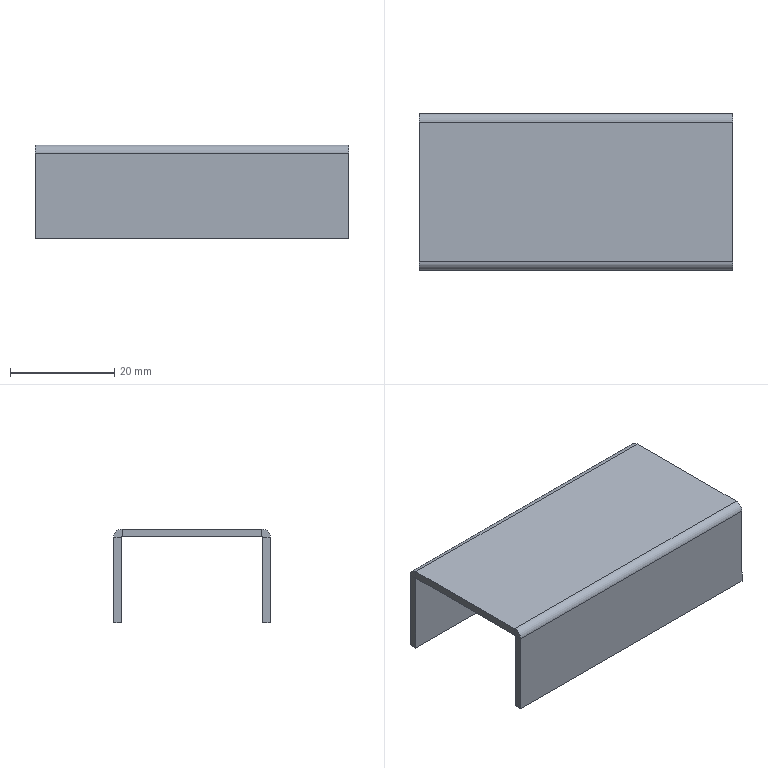Part | SolidWorks | features EdgeFlange 1, FlatPattern 1, SMBaseFlange 1, SheetMetal 1 | 1 solid | 22 faces | box 60 x 30 x 18 mm | volume 5604 mm3 | plane 18 | cylinder 4 | commonest cylinder face diameters 0.2 x2 3.2 x2
STEP:
#1=CARTESIAN_POINT('',(30.,13.4,-1.5));
#2=VERTEX_POINT('',#1);
#3=CARTESIAN_POINT('',(-30.,13.4,-1.5));
#4=VERTEX_POINT('',#3);
#5=CARTESIAN_POINT('',(30.,13.4,-1.5));
#6=DIRECTION('',(-1.,0.,0.));
#7=VECTOR('',#6,1000.);
#8=LINE('',#5,#7);
#9=EDGE_CURVE('',#2,#4,#8,.T.);
#10=ORIENTED_EDGE('',*,*,#9,.F.);
#11=CARTESIAN_POINT('',(30.,-13.4,-1.5));
#12=VERTEX_POINT('',#11);
#13=CARTESIAN_POINT('',(30.,15.,-1.5));
#14=DIRECTION('',(0.,1.,0.));
#15=VECTOR('',#14,1000.);
#16=LINE('',#13,#15);
#17=EDGE_CURVE('',#12,#2,#16,.T.);
#18=ORIENTED_EDGE('',*,*,#17,.F.);
#19=CARTESIAN_POINT('',(-30.,-13.4,-1.5));
#20=VERTEX_POINT('',#19);
#21=CARTESIAN_POINT('',(-30.,-13.4,-1.5));
#22=DIRECTION('',(1.,0.,0.));
#23=VECTOR('',#22,1000.);
#24=LINE('',#21,#23);
#25=EDGE_CURVE('',#20,#12,#24,.T.);
#26=ORIENTED_EDGE('',*,*,#25,.F.);
#27=CARTESIAN_POINT('',(-30.,15.,-1.5));
#28=DIRECTION('',(0.,-1.,0.));
#29=VECTOR('',#28,1000.);
#30=LINE('',#27,#29);
#31=EDGE_CURVE('',#4,#20,#30,.T.);
#32=ORIENTED_EDGE('',*,*,#31,.F.);
#33=EDGE_LOOP('',(#10,#18,#26,#32));
#34=FACE_OUTER_BOUND('',#33,.T.);
#35=CARTESIAN_POINT('',(0.,0.,-1.5));
#36=DIRECTION('',(0.,0.,1.));
#37=DIRECTION('',(1.,0.,0.));
#38=AXIS2_PLACEMENT_3D('',#35,#36,#37);
#39=PLANE('',#38);
#40=ADVANCED_FACE('',(#34),#39,.F.);
#41=CARTESIAN_POINT('',(30.,-13.4,0.));
#42=VERTEX_POINT('',#41);
#43=CARTESIAN_POINT('',(30.,13.4,0.));
#44=VERTEX_POINT('',#43);
#45=CARTESIAN_POINT('',(30.,15.,0.));
#46=DIRECTION('',(0.,1.,0.));
#47=VECTOR('',#46,1000.);
#48=LINE('',#45,#47);
#49=EDGE_CURVE('',#42,#44,#48,.T.);
#50=ORIENTED_EDGE('',*,*,#49,.T.);
#51=CARTESIAN_POINT('',(-30.,13.4,0.));
#52=VERTEX_POINT('',#51);
#53=CARTESIAN_POINT('',(30.,13.4,0.));
#54=DIRECTION('',(-1.,0.,0.));
#55=VECTOR('',#54,1000.);
#56=LINE('',#53,#55);
#57=EDGE_CURVE('',#44,#52,#56,.T.);
#58=ORIENTED_EDGE('',*,*,#57,.T.);
#59=CARTESIAN_POINT('',(-30.,-13.4,0.));
#60=VERTEX_POINT('',#59);
#61=CARTESIAN_POINT('',(-30.,15.,0.));
#62=DIRECTION('',(0.,-1.,0.));
#63=VECTOR('',#62,1000.);
#64=LINE('',#61,#63);
#65=EDGE_CURVE('',#52,#60,#64,.T.);
#66=ORIENTED_EDGE('',*,*,#65,.T.);
#67=CARTESIAN_POINT('',(-30.,-13.4,0.));
#68=DIRECTION('',(1.,0.,0.));
#69=VECTOR('',#68,1000.);
#70=LINE('',#67,#69);
#71=EDGE_CURVE('',#60,#42,#70,.T.);
#72=ORIENTED_EDGE('',*,*,#71,.T.);
#73=EDGE_LOOP('',(#50,#58,#66,#72));
#74=FACE_OUTER_BOUND('',#73,.T.);
#75=CARTESIAN_POINT('',(0.,0.,0.));
#76=DIRECTION('',(0.,0.,1.));
#77=DIRECTION('',(1.,0.,0.));
#78=AXIS2_PLACEMENT_3D('',#75,#76,#77);
#79=PLANE('',#78);
#80=ADVANCED_FACE('',(#74),#79,.T.);
#81=ORIENTED_EDGE('',*,*,#17,.T.);
#82=CARTESIAN_POINT('',(30.,13.4,-1.5));
#83=DIRECTION('',(0.,0.,1.));
#84=VECTOR('',#83,1000.);
#85=LINE('',#82,#84);
#86=EDGE_CURVE('',#2,#44,#85,.T.);
#87=ORIENTED_EDGE('',*,*,#86,.T.);
#88=ORIENTED_EDGE('',*,*,#49,.F.);
#89=CARTESIAN_POINT('',(30.,-13.4,-1.5));
#90=DIRECTION('',(0.,0.,1.));
#91=VECTOR('',#90,1000.);
#92=LINE('',#89,#91);
#93=EDGE_CURVE('',#12,#42,#92,.T.);
#94=ORIENTED_EDGE('',*,*,#93,.F.);
#95=EDGE_LOOP('',(#81,#87,#88,#94));
#96=FACE_OUTER_BOUND('',#95,.T.);
#97=CARTESIAN_POINT('',(30.,15.,-1.5));
#98=DIRECTION('',(1.,0.,0.));
#99=DIRECTION('',(0.,0.,-1.));
#100=AXIS2_PLACEMENT_3D('',#97,#98,#99);
#101=PLANE('',#100);
#102=ADVANCED_FACE('',(#96),#101,.T.);
#103=CARTESIAN_POINT('',(-30.,13.4,-1.5));
#104=DIRECTION('',(0.,0.,1.));
#105=VECTOR('',#104,1000.);
#106=LINE('',#103,#105);
#107=EDGE_CURVE('',#4,#52,#106,.T.);
#108=ORIENTED_EDGE('',*,*,#107,.F.);
#109=ORIENTED_EDGE('',*,*,#31,.T.);
#110=CARTESIAN_POINT('',(-30.,-13.4,-1.5));
#111=DIRECTION('',(0.,0.,1.));
#112=VECTOR('',#111,1000.);
#113=LINE('',#110,#112);
#114=EDGE_CURVE('',#20,#60,#113,.T.);
#115=ORIENTED_EDGE('',*,*,#114,.T.);
#116=ORIENTED_EDGE('',*,*,#65,.F.);
#117=EDGE_LOOP('',(#108,#109,#115,#116));
#118=FACE_OUTER_BOUND('',#117,.T.);
#119=CARTESIAN_POINT('',(-30.,15.,-1.5));
#120=DIRECTION('',(-1.,0.,0.));
#121=DIRECTION('',(0.,0.,1.));
#122=AXIS2_PLACEMENT_3D('',#119,#120,#121);
#123=PLANE('',#122);
#124=ADVANCED_FACE('',(#118),#123,.T.);
#125=CARTESIAN_POINT('',(30.,-13.5,-1.6));
#126=VERTEX_POINT('',#125);
#127=CARTESIAN_POINT('',(30.,-15.,-1.6));
#128=VERTEX_POINT('',#127);
#129=CARTESIAN_POINT('',(30.,-15.,-1.6));
#130=DIRECTION('',(0.,-1.,0.));
#131=VECTOR('',#130,1000.);
#132=LINE('',#129,#131);
#133=EDGE_CURVE('',#126,#128,#132,.T.);
#134=ORIENTED_EDGE('',*,*,#133,.F.);
#135=CARTESIAN_POINT('',(30.,-13.4,-1.6));
#136=DIRECTION('',(1.,0.,0.));
#137=DIRECTION('',(0.,0.,1.));
#138=AXIS2_PLACEMENT_3D('',#135,#136,#137);
#139=CIRCLE('',#138,0.1);
#140=EDGE_CURVE('',#12,#126,#139,.T.);
#141=ORIENTED_EDGE('',*,*,#140,.F.);
#142=ORIENTED_EDGE('',*,*,#93,.T.);
#143=CARTESIAN_POINT('',(30.,-13.4,-1.6));
#144=DIRECTION('',(1.,0.,0.));
#145=DIRECTION('',(0.,0.,1.));
#146=AXIS2_PLACEMENT_3D('',#143,#144,#145);
#147=CIRCLE('',#146,1.6);
#148=EDGE_CURVE('',#42,#128,#147,.T.);
#149=ORIENTED_EDGE('',*,*,#148,.T.);
#150=EDGE_LOOP('',(#134,#141,#142,#149));
#151=FACE_OUTER_BOUND('',#150,.T.);
#152=CARTESIAN_POINT('',(30.,-13.4,-1.6));
#153=DIRECTION('',(1.,0.,0.));
#154=DIRECTION('',(0.,0.,-1.));
#155=AXIS2_PLACEMENT_3D('',#152,#153,#154);
#156=PLANE('',#155);
#157=ADVANCED_FACE('',(#151),#156,.T.);
#158=CARTESIAN_POINT('',(-30.,-13.5,-1.6));
#159=VERTEX_POINT('',#158);
#160=CARTESIAN_POINT('',(-30.,-13.4,-1.6));
#161=DIRECTION('',(-1.,0.,0.));
#162=DIRECTION('',(0.,0.,1.));
#163=AXIS2_PLACEMENT_3D('',#160,#161,#162);
#164=CIRCLE('',#163,0.1);
#165=EDGE_CURVE('',#159,#20,#164,.T.);
#166=ORIENTED_EDGE('',*,*,#165,.F.);
#167=CARTESIAN_POINT('',(-30.,-15.,-1.6));
#168=VERTEX_POINT('',#167);
#169=CARTESIAN_POINT('',(-30.,-13.5,-1.6));
#170=DIRECTION('',(0.,-1.,0.));
#171=VECTOR('',#170,1000.);
#172=LINE('',#169,#171);
#173=EDGE_CURVE('',#159,#168,#172,.T.);
#174=ORIENTED_EDGE('',*,*,#173,.T.);
#175=CARTESIAN_POINT('',(-30.,-13.4,-1.6));
#176=DIRECTION('',(-1.,0.,0.));
#177=DIRECTION('',(0.,0.,1.));
#178=AXIS2_PLACEMENT_3D('',#175,#176,#177);
#179=CIRCLE('',#178,1.6);
#180=EDGE_CURVE('',#168,#60,#179,.T.);
#181=ORIENTED_EDGE('',*,*,#180,.T.);
#182=ORIENTED_EDGE('',*,*,#114,.F.);
#183=EDGE_LOOP('',(#166,#174,#181,#182));
#184=FACE_OUTER_BOUND('',#183,.T.);
#185=CARTESIAN_POINT('',(-30.,-13.4,-1.6));
#186=DIRECTION('',(1.,0.,0.));
#187=DIRECTION('',(0.,0.,-1.));
#188=AXIS2_PLACEMENT_3D('',#185,#186,#187);
#189=PLANE('',#188);
#190=ADVANCED_FACE('',(#184),#189,.F.);
#191=ORIENTED_EDGE('',*,*,#71,.F.);
#192=ORIENTED_EDGE('',*,*,#180,.F.);
#193=CARTESIAN_POINT('',(0.,-15.,-1.6));
#194=DIRECTION('',(-1.,0.,0.));
#195=VECTOR('',#194,1000.);
#196=LINE('',#193,#195);
#197=EDGE_CURVE('',#128,#168,#196,.T.);
#198=ORIENTED_EDGE('',*,*,#197,.F.);
#199=ORIENTED_EDGE('',*,*,#148,.F.);
#200=EDGE_LOOP('',(#191,#192,#198,#199));
#201=FACE_OUTER_BOUND('',#200,.T.);
#202=CARTESIAN_POINT('',(-30.,-13.4,-1.6));
#203=DIRECTION('',(-1.,0.,0.));
#204=DIRECTION('',(0.,-1.,0.));
#205=AXIS2_PLACEMENT_3D('',#202,#203,#204);
#206=CYLINDRICAL_SURFACE('',#205,1.6);
#207=ADVANCED_FACE('',(#201),#206,.T.);
#208=ORIENTED_EDGE('',*,*,#25,.T.);
#209=ORIENTED_EDGE('',*,*,#140,.T.);
#210=CARTESIAN_POINT('',(30.,-13.5,-1.6));
#211=DIRECTION('',(-1.,0.,0.));
#212=VECTOR('',#211,1000.);
#213=LINE('',#210,#212);
#214=EDGE_CURVE('',#126,#159,#213,.T.);
#215=ORIENTED_EDGE('',*,*,#214,.T.);
#216=ORIENTED_EDGE('',*,*,#165,.T.);
#217=EDGE_LOOP('',(#208,#209,#215,#216));
#218=FACE_OUTER_BOUND('',#217,.T.);
#219=CARTESIAN_POINT('',(-30.,-13.4,-1.6));
#220=DIRECTION('',(-1.,0.,0.));
#221=DIRECTION('',(0.,-1.,0.));
#222=AXIS2_PLACEMENT_3D('',#219,#220,#221);
#223=CYLINDRICAL_SURFACE('',#222,0.1);
#224=ADVANCED_FACE('',(#218),#223,.F.);
#225=CARTESIAN_POINT('',(-30.,-15.,-18.));
#226=VERTEX_POINT('',#225);
#227=CARTESIAN_POINT('',(-30.,-15.,-1.5));
#228=DIRECTION('',(0.,0.,1.));
#229=VECTOR('',#228,1000.);
#230=LINE('',#227,#229);
#231=EDGE_CURVE('',#226,#168,#230,.T.);
#232=ORIENTED_EDGE('',*,*,#231,.T.);
#233=ORIENTED_EDGE('',*,*,#173,.F.);
#234=CARTESIAN_POINT('',(-30.,-13.5,-18.));
#235=VERTEX_POINT('',#234);
#236=CARTESIAN_POINT('',(-30.,-13.5,0.));
#237=DIRECTION('',(0.,0.,1.));
#238=VECTOR('',#237,1000.);
#239=LINE('',#236,#238);
#240=EDGE_CURVE('',#235,#159,#239,.T.);
#241=ORIENTED_EDGE('',*,*,#240,.F.);
#242=CARTESIAN_POINT('',(-30.,-15.,-18.));
#243=DIRECTION('',(0.,1.,0.));
#244=VECTOR('',#243,1000.);
#245=LINE('',#242,#244);
#246=EDGE_CURVE('',#226,#235,#245,.T.);
#247=ORIENTED_EDGE('',*,*,#246,.F.);
#248=EDGE_LOOP('',(#232,#233,#241,#247));
#249=FACE_OUTER_BOUND('',#248,.T.);
#250=CARTESIAN_POINT('',(-30.,-15.,-1.5));
#251=DIRECTION('',(-1.,0.,0.));
#252=DIRECTION('',(0.,0.,1.));
#253=AXIS2_PLACEMENT_3D('',#250,#251,#252);
#254=PLANE('',#253);
#255=ADVANCED_FACE('',(#249),#254,.T.);
#256=CARTESIAN_POINT('',(30.,-13.5,-18.));
#257=VERTEX_POINT('',#256);
#258=CARTESIAN_POINT('',(30.,-13.5,0.));
#259=DIRECTION('',(0.,0.,-1.));
#260=VECTOR('',#259,1000.);
#261=LINE('',#258,#260);
#262=EDGE_CURVE('',#126,#257,#261,.T.);
#263=ORIENTED_EDGE('',*,*,#262,.F.);
#264=ORIENTED_EDGE('',*,*,#133,.T.);
#265=CARTESIAN_POINT('',(30.,-15.,-18.));
#266=VERTEX_POINT('',#265);
#267=CARTESIAN_POINT('',(30.,-15.,-18.));
#268=DIRECTION('',(0.,0.,-1.));
#269=VECTOR('',#268,1000.);
#270=LINE('',#267,#269);
#271=EDGE_CURVE('',#128,#266,#270,.T.);
#272=ORIENTED_EDGE('',*,*,#271,.T.);
#273=CARTESIAN_POINT('',(30.,-15.,-18.));
#274=DIRECTION('',(0.,1.,0.));
#275=VECTOR('',#274,1000.);
#276=LINE('',#273,#275);
#277=EDGE_CURVE('',#266,#257,#276,.T.);
#278=ORIENTED_EDGE('',*,*,#277,.T.);
#279=EDGE_LOOP('',(#263,#264,#272,#278));
#280=FACE_OUTER_BOUND('',#279,.T.);
#281=CARTESIAN_POINT('',(30.,-15.,-18.));
#282=DIRECTION('',(1.,0.,0.));
#283=DIRECTION('',(0.,0.,-1.));
#284=AXIS2_PLACEMENT_3D('',#281,#282,#283);
#285=PLANE('',#284);
#286=ADVANCED_FACE('',(#280),#285,.T.);
#287=ORIENTED_EDGE('',*,*,#271,.F.);
#288=ORIENTED_EDGE('',*,*,#197,.T.);
#289=ORIENTED_EDGE('',*,*,#231,.F.);
#290=CARTESIAN_POINT('',(-30.,-15.,-18.));
#291=DIRECTION('',(-1.,0.,0.));
#292=VECTOR('',#291,1000.);
#293=LINE('',#290,#292);
#294=EDGE_CURVE('',#266,#226,#293,.T.);
#295=ORIENTED_EDGE('',*,*,#294,.F.);
#296=EDGE_LOOP('',(#287,#288,#289,#295));
#297=FACE_OUTER_BOUND('',#296,.T.);
#298=CARTESIAN_POINT('',(0.,-15.,0.));
#299=DIRECTION('',(0.,-1.,0.));
#300=DIRECTION('',(0.,0.,-1.));
#301=AXIS2_PLACEMENT_3D('',#298,#299,#300);
#302=PLANE('',#301);
#303=ADVANCED_FACE('',(#297),#302,.T.);
#304=ORIENTED_EDGE('',*,*,#214,.F.);
#305=ORIENTED_EDGE('',*,*,#262,.T.);
#306=CARTESIAN_POINT('',(0.,-13.5,-18.));
#307=DIRECTION('',(-1.,0.,0.));
#308=VECTOR('',#307,1000.);
#309=LINE('',#306,#308);
#310=EDGE_CURVE('',#257,#235,#309,.T.);
#311=ORIENTED_EDGE('',*,*,#310,.T.);
#312=ORIENTED_EDGE('',*,*,#240,.T.);
#313=EDGE_LOOP('',(#304,#305,#311,#312));
#314=FACE_OUTER_BOUND('',#313,.T.);
#315=CARTESIAN_POINT('',(0.,-13.5,0.));
#316=DIRECTION('',(0.,-1.,0.));
#317=DIRECTION('',(0.,0.,-1.));
#318=AXIS2_PLACEMENT_3D('',#315,#316,#317);
#319=PLANE('',#318);
#320=ADVANCED_FACE('',(#314),#319,.F.);
#321=ORIENTED_EDGE('',*,*,#310,.F.);
#322=ORIENTED_EDGE('',*,*,#277,.F.);
#323=ORIENTED_EDGE('',*,*,#294,.T.);
#324=ORIENTED_EDGE('',*,*,#246,.T.);
#325=EDGE_LOOP('',(#321,#322,#323,#324));
#326=FACE_OUTER_BOUND('',#325,.T.);
#327=CARTESIAN_POINT('',(-30.,-15.,-18.));
#328=DIRECTION('',(0.,0.,-1.));
#329=DIRECTION('',(0.,1.,0.));
#330=AXIS2_PLACEMENT_3D('',#327,#328,#329);
#331=PLANE('',#330);
#332=ADVANCED_FACE('',(#326),#331,.T.);
#333=CARTESIAN_POINT('',(-30.,13.5,-1.6));
#334=VERTEX_POINT('',#333);
#335=CARTESIAN_POINT('',(-30.,15.,-1.6));
#336=VERTEX_POINT('',#335);
#337=CARTESIAN_POINT('',(-30.,15.,-1.6));
#338=DIRECTION('',(0.,1.,0.));
#339=VECTOR('',#338,1000.);
#340=LINE('',#337,#339);
#341=EDGE_CURVE('',#334,#336,#340,.T.);
#342=ORIENTED_EDGE('',*,*,#341,.F.);
#343=CARTESIAN_POINT('',(-30.,13.4,-1.6));
#344=DIRECTION('',(-1.,0.,0.));
#345=DIRECTION('',(0.,0.,-1.));
#346=AXIS2_PLACEMENT_3D('',#343,#344,#345);
#347=CIRCLE('',#346,0.1);
#348=EDGE_CURVE('',#4,#334,#347,.T.);
#349=ORIENTED_EDGE('',*,*,#348,.F.);
#350=ORIENTED_EDGE('',*,*,#107,.T.);
#351=CARTESIAN_POINT('',(-30.,13.4,-1.6));
#352=DIRECTION('',(-1.,0.,0.));
#353=DIRECTION('',(0.,0.,-1.));
#354=AXIS2_PLACEMENT_3D('',#351,#352,#353);
#355=CIRCLE('',#354,1.6);
#356=EDGE_CURVE('',#52,#336,#355,.T.);
#357=ORIENTED_EDGE('',*,*,#356,.T.);
#358=EDGE_LOOP('',(#342,#349,#350,#357));
#359=FACE_OUTER_BOUND('',#358,.T.);
#360=CARTESIAN_POINT('',(-30.,13.4,-1.6));
#361=DIRECTION('',(-1.,0.,0.));
#362=DIRECTION('',(0.,0.,1.));
#363=AXIS2_PLACEMENT_3D('',#360,#361,#362);
#364=PLANE('',#363);
#365=ADVANCED_FACE('',(#359),#364,.T.);
#366=CARTESIAN_POINT('',(30.,13.5,-1.6));
#367=VERTEX_POINT('',#366);
#368=CARTESIAN_POINT('',(30.,13.4,-1.6));
#369=DIRECTION('',(1.,0.,0.));
#370=DIRECTION('',(0.,0.,-1.));
#371=AXIS2_PLACEMENT_3D('',#368,#369,#370);
#372=CIRCLE('',#371,0.1);
#373=EDGE_CURVE('',#367,#2,#372,.T.);
#374=ORIENTED_EDGE('',*,*,#373,.F.);
#375=CARTESIAN_POINT('',(30.,15.,-1.6));
#376=VERTEX_POINT('',#375);
#377=CARTESIAN_POINT('',(30.,13.5,-1.6));
#378=DIRECTION('',(0.,1.,0.));
#379=VECTOR('',#378,1000.);
#380=LINE('',#377,#379);
#381=EDGE_CURVE('',#367,#376,#380,.T.);
#382=ORIENTED_EDGE('',*,*,#381,.T.);
#383=CARTESIAN_POINT('',(30.,13.4,-1.6));
#384=DIRECTION('',(1.,0.,0.));
#385=DIRECTION('',(0.,0.,-1.));
#386=AXIS2_PLACEMENT_3D('',#383,#384,#385);
#387=CIRCLE('',#386,1.6);
#388=EDGE_CURVE('',#376,#44,#387,.T.);
#389=ORIENTED_EDGE('',*,*,#388,.T.);
#390=ORIENTED_EDGE('',*,*,#86,.F.);
#391=EDGE_LOOP('',(#374,#382,#389,#390));
#392=FACE_OUTER_BOUND('',#391,.T.);
#393=CARTESIAN_POINT('',(30.,13.4,-1.6));
#394=DIRECTION('',(-1.,0.,0.));
#395=DIRECTION('',(0.,0.,1.));
#396=AXIS2_PLACEMENT_3D('',#393,#394,#395);
#397=PLANE('',#396);
#398=ADVANCED_FACE('',(#392),#397,.F.);
#399=ORIENTED_EDGE('',*,*,#57,.F.);
#400=ORIENTED_EDGE('',*,*,#388,.F.);
#401=CARTESIAN_POINT('',(-30.,15.,-1.6));
#402=DIRECTION('',(-1.,0.,0.));
#403=VECTOR('',#402,1000.);
#404=LINE('',#401,#403);
#405=EDGE_CURVE('',#376,#336,#404,.T.);
#406=ORIENTED_EDGE('',*,*,#405,.T.);
#407=ORIENTED_EDGE('',*,*,#356,.F.);
#408=EDGE_LOOP('',(#399,#400,#406,#407));
#409=FACE_OUTER_BOUND('',#408,.T.);
#410=CARTESIAN_POINT('',(30.,13.4,-1.6));
#411=DIRECTION('',(1.,0.,0.));
#412=DIRECTION('',(0.,1.,0.));
#413=AXIS2_PLACEMENT_3D('',#410,#411,#412);
#414=CYLINDRICAL_SURFACE('',#413,1.6);
#415=ADVANCED_FACE('',(#409),#414,.T.);
#416=ORIENTED_EDGE('',*,*,#9,.T.);
#417=ORIENTED_EDGE('',*,*,#348,.T.);
#418=CARTESIAN_POINT('',(-30.,13.5,-1.6));
#419=DIRECTION('',(1.,0.,0.));
#420=VECTOR('',#419,1000.);
#421=LINE('',#418,#420);
#422=EDGE_CURVE('',#334,#367,#421,.T.);
#423=ORIENTED_EDGE('',*,*,#422,.T.);
#424=ORIENTED_EDGE('',*,*,#373,.T.);
#425=EDGE_LOOP('',(#416,#417,#423,#424));
#426=FACE_OUTER_BOUND('',#425,.T.);
#427=CARTESIAN_POINT('',(30.,13.4,-1.6));
#428=DIRECTION('',(1.,0.,0.));
#429=DIRECTION('',(0.,1.,0.));
#430=AXIS2_PLACEMENT_3D('',#427,#428,#429);
#431=CYLINDRICAL_SURFACE('',#430,0.1);
#432=ADVANCED_FACE('',(#426),#431,.F.);
#433=CARTESIAN_POINT('',(-30.,13.5,-18.));
#434=VERTEX_POINT('',#433);
#435=CARTESIAN_POINT('',(-30.,13.5,0.));
#436=DIRECTION('',(0.,0.,-1.));
#437=VECTOR('',#436,1000.);
#438=LINE('',#435,#437);
#439=EDGE_CURVE('',#334,#434,#438,.T.);
#440=ORIENTED_EDGE('',*,*,#439,.F.);
#441=ORIENTED_EDGE('',*,*,#341,.T.);
#442=CARTESIAN_POINT('',(-30.,15.,-18.));
#443=VERTEX_POINT('',#442);
#444=CARTESIAN_POINT('',(-30.,15.,-1.5));
#445=DIRECTION('',(0.,0.,-1.));
#446=VECTOR('',#445,1000.);
#447=LINE('',#444,#446);
#448=EDGE_CURVE('',#336,#443,#447,.T.);
#449=ORIENTED_EDGE('',*,*,#448,.T.);
#450=CARTESIAN_POINT('',(-30.,15.,-18.));
#451=DIRECTION('',(0.,-1.,0.));
#452=VECTOR('',#451,1000.);
#453=LINE('',#450,#452);
#454=EDGE_CURVE('',#443,#434,#453,.T.);
#455=ORIENTED_EDGE('',*,*,#454,.T.);
#456=EDGE_LOOP('',(#440,#441,#449,#455));
#457=FACE_OUTER_BOUND('',#456,.T.);
#458=CARTESIAN_POINT('',(-30.,15.,-1.5));
#459=DIRECTION('',(-1.,0.,0.));
#460=DIRECTION('',(0.,0.,1.));
#461=AXIS2_PLACEMENT_3D('',#458,#459,#460);
#462=PLANE('',#461);
#463=ADVANCED_FACE('',(#457),#462,.T.);
#464=CARTESIAN_POINT('',(30.,15.,-18.));
#465=VERTEX_POINT('',#464);
#466=CARTESIAN_POINT('',(30.,15.,-18.));
#467=DIRECTION('',(0.,0.,1.));
#468=VECTOR('',#467,1000.);
#469=LINE('',#466,#468);
#470=EDGE_CURVE('',#465,#376,#469,.T.);
#471=ORIENTED_EDGE('',*,*,#470,.T.);
#472=ORIENTED_EDGE('',*,*,#381,.F.);
#473=CARTESIAN_POINT('',(30.,13.5,-18.));
#474=VERTEX_POINT('',#473);
#475=CARTESIAN_POINT('',(30.,13.5,0.));
#476=DIRECTION('',(0.,0.,1.));
#477=VECTOR('',#476,1000.);
#478=LINE('',#475,#477);
#479=EDGE_CURVE('',#474,#367,#478,.T.);
#480=ORIENTED_EDGE('',*,*,#479,.F.);
#481=CARTESIAN_POINT('',(30.,15.,-18.));
#482=DIRECTION('',(0.,-1.,0.));
#483=VECTOR('',#482,1000.);
#484=LINE('',#481,#483);
#485=EDGE_CURVE('',#465,#474,#484,.T.);
#486=ORIENTED_EDGE('',*,*,#485,.F.);
#487=EDGE_LOOP('',(#471,#472,#480,#486));
#488=FACE_OUTER_BOUND('',#487,.T.);
#489=CARTESIAN_POINT('',(30.,15.,-18.));
#490=DIRECTION('',(1.,0.,0.));
#491=DIRECTION('',(0.,0.,-1.));
#492=AXIS2_PLACEMENT_3D('',#489,#490,#491);
#493=PLANE('',#492);
#494=ADVANCED_FACE('',(#488),#493,.T.);
#495=ORIENTED_EDGE('',*,*,#405,.F.);
#496=ORIENTED_EDGE('',*,*,#470,.F.);
#497=CARTESIAN_POINT('',(-30.,15.,-18.));
#498=DIRECTION('',(1.,0.,0.));
#499=VECTOR('',#498,1000.);
#500=LINE('',#497,#499);
#501=EDGE_CURVE('',#443,#465,#500,.T.);
#502=ORIENTED_EDGE('',*,*,#501,.F.);
#503=ORIENTED_EDGE('',*,*,#448,.F.);
#504=EDGE_LOOP('',(#495,#496,#502,#503));
#505=FACE_OUTER_BOUND('',#504,.T.);
#506=CARTESIAN_POINT('',(0.,15.,0.));
#507=DIRECTION('',(0.,-1.,0.));
#508=DIRECTION('',(0.,0.,-1.));
#509=AXIS2_PLACEMENT_3D('',#506,#507,#508);
#510=PLANE('',#509);
#511=ADVANCED_FACE('',(#505),#510,.F.);
#512=ORIENTED_EDGE('',*,*,#479,.T.);
#513=ORIENTED_EDGE('',*,*,#422,.F.);
#514=ORIENTED_EDGE('',*,*,#439,.T.);
#515=CARTESIAN_POINT('',(0.,13.5,-18.));
#516=DIRECTION('',(1.,0.,0.));
#517=VECTOR('',#516,1000.);
#518=LINE('',#515,#517);
#519=EDGE_CURVE('',#434,#474,#518,.T.);
#520=ORIENTED_EDGE('',*,*,#519,.T.);
#521=EDGE_LOOP('',(#512,#513,#514,#520));
#522=FACE_OUTER_BOUND('',#521,.T.);
#523=CARTESIAN_POINT('',(0.,13.5,0.));
#524=DIRECTION('',(0.,-1.,0.));
#525=DIRECTION('',(0.,0.,-1.));
#526=AXIS2_PLACEMENT_3D('',#523,#524,#525);
#527=PLANE('',#526);
#528=ADVANCED_FACE('',(#522),#527,.T.);
#529=ORIENTED_EDGE('',*,*,#519,.F.);
#530=ORIENTED_EDGE('',*,*,#454,.F.);
#531=ORIENTED_EDGE('',*,*,#501,.T.);
#532=ORIENTED_EDGE('',*,*,#485,.T.);
#533=EDGE_LOOP('',(#529,#530,#531,#532));
#534=FACE_OUTER_BOUND('',#533,.T.);
#535=CARTESIAN_POINT('',(-30.,15.,-18.));
#536=DIRECTION('',(0.,0.,-1.));
#537=DIRECTION('',(0.,1.,0.));
#538=AXIS2_PLACEMENT_3D('',#535,#536,#537);
#539=PLANE('',#538);
#540=ADVANCED_FACE('',(#534),#539,.T.);
#541=CLOSED_SHELL('',(#40,#80,#102,#124,#157,#190,#207,#224,#255,#286,#303,#320,#332,#365,#398,#415,#432,#463,#494,#511,#528,#540));
#542=MANIFOLD_SOLID_BREP('',#541);
#543=CARTESIAN_POINT('',(0.,0.,0.));
#544=DIRECTION('',(0.,0.,1.));
#545=DIRECTION('',(1.,0.,0.));
#546=AXIS2_PLACEMENT_3D('',#543,#544,#545);
#547=(LENGTH_UNIT()NAMED_UNIT(*)SI_UNIT(.MILLI.,.METRE.));
#548=UNCERTAINTY_MEASURE_WITH_UNIT(LENGTH_MEASURE(0.00001),#547,'','');
#549=(NAMED_UNIT(*)PLANE_ANGLE_UNIT()SI_UNIT($,.RADIAN.));
#550=(NAMED_UNIT(*)SI_UNIT($,.STERADIAN.)SOLID_ANGLE_UNIT());
#551=(GEOMETRIC_REPRESENTATION_CONTEXT(3)GLOBAL_UNCERTAINTY_ASSIGNED_CONTEXT((#548))GLOBAL_UNIT_ASSIGNED_CONTEXT((#547,#549,#550))REPRESENTATION_CONTEXT('',''));
#552=ADVANCED_BREP_SHAPE_REPRESENTATION('',(#542,#546),#551);